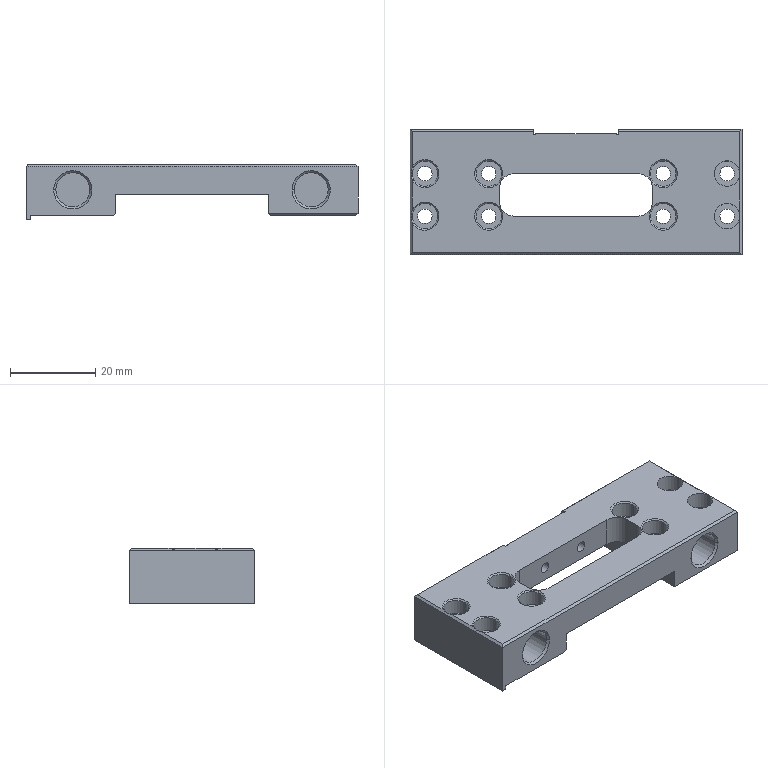Part | NX | 1 solid | 119 faces | box 78 x 29.4 x 13 mm | volume 16135 mm3 | cylinder 48 | plane 43 | cone 28 | commonest cylinder face diameters 3.4 x16 6 x16 2.5 x8 7 x4 8 x4